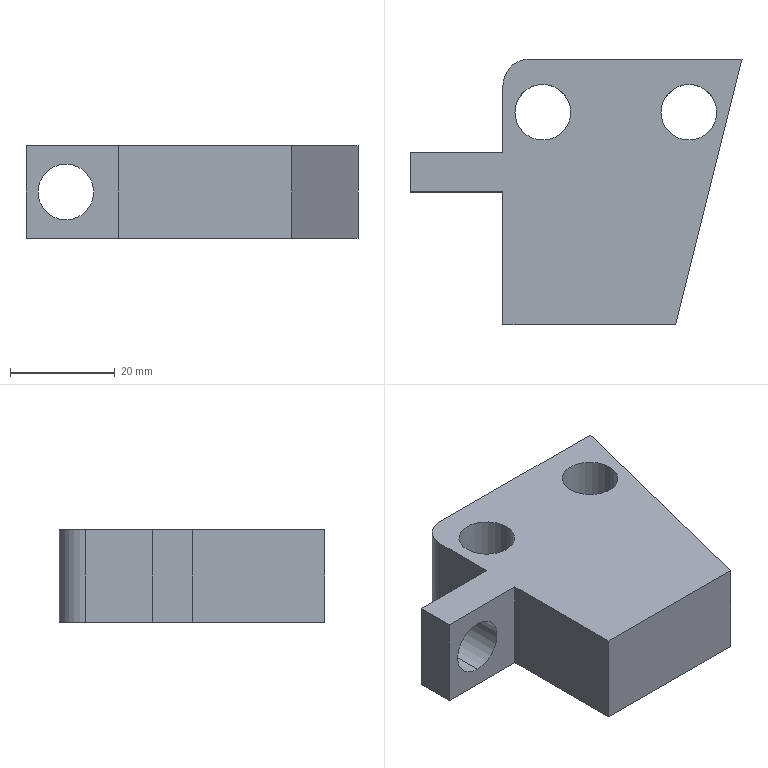Part | SolidWorks | features Extrusion 1, Fillet 1, ICE 1, Scale 1 | 1 solid | 17 faces | box 63.5 x 50.8 x 17.78 mm | volume 34011 mm3 | plane 10 | cylinder 7 | commonest cylinder face diameters 10.668 x6 10.16 x1
STEP:
#1=CARTESIAN_POINT('',(-10.16,25.4,3.556));
#2=VERTEX_POINT('',#1);
#3=CARTESIAN_POINT('',(-10.16,25.4,14.224));
#4=VERTEX_POINT('',#3);
#5=CARTESIAN_POINT('',(-10.16,25.4,8.89));
#6=DIRECTION('',(0.,1.,0.));
#7=DIRECTION('',(-1.,0.,0.));
#8=AXIS2_PLACEMENT_3D('',#5,#6,#7);
#9=CIRCLE('',#8,5.334);
#10=EDGE_CURVE('',#2,#4,#9,.T.);
#11=ORIENTED_EDGE('',*,*,#10,.F.);
#12=CARTESIAN_POINT('',(-10.16,33.02,3.556));
#13=VERTEX_POINT('',#12);
#14=CARTESIAN_POINT('',(-10.16,0.,3.556));
#15=DIRECTION('',(0.,1.,0.));
#16=VECTOR('',#15,1000.);
#17=LINE('',#14,#16);
#18=EDGE_CURVE('',#2,#13,#17,.T.);
#19=ORIENTED_EDGE('',*,*,#18,.T.);
#20=CARTESIAN_POINT('',(-10.16,33.02,14.224));
#21=VERTEX_POINT('',#20);
#22=CARTESIAN_POINT('',(-10.16,33.02,8.89));
#23=DIRECTION('',(0.,1.,0.));
#24=DIRECTION('',(0.,0.,1.));
#25=AXIS2_PLACEMENT_3D('',#22,#23,#24);
#26=CIRCLE('',#25,5.334);
#27=EDGE_CURVE('',#13,#21,#26,.T.);
#28=ORIENTED_EDGE('',*,*,#27,.T.);
#29=CARTESIAN_POINT('',(-10.16,0.,14.224));
#30=DIRECTION('',(0.,1.,0.));
#31=VECTOR('',#30,1000.);
#32=LINE('',#29,#31);
#33=EDGE_CURVE('',#4,#21,#32,.T.);
#34=ORIENTED_EDGE('',*,*,#33,.F.);
#35=EDGE_LOOP('',(#11,#19,#28,#34));
#36=FACE_OUTER_BOUND('',#35,.T.);
#37=CARTESIAN_POINT('',(-10.16,0.,8.89));
#38=DIRECTION('',(0.,1.,0.));
#39=DIRECTION('',(0.,0.,1.));
#40=AXIS2_PLACEMENT_3D('',#37,#38,#39);
#41=CYLINDRICAL_SURFACE('',#40,5.334);
#42=ADVANCED_FACE('',(#36),#41,.F.);
#43=CARTESIAN_POINT('',(30.226,40.64,17.78));
#44=VERTEX_POINT('',#43);
#45=CARTESIAN_POINT('',(40.894,40.64,17.78));
#46=VERTEX_POINT('',#45);
#47=CARTESIAN_POINT('',(35.56,40.64,17.78));
#48=DIRECTION('',(0.,0.,1.));
#49=DIRECTION('',(1.,0.,0.));
#50=AXIS2_PLACEMENT_3D('',#47,#48,#49);
#51=CIRCLE('',#50,5.334);
#52=EDGE_CURVE('',#44,#46,#51,.T.);
#53=ORIENTED_EDGE('',*,*,#52,.T.);
#54=CARTESIAN_POINT('',(40.894,40.64,0.));
#55=VERTEX_POINT('',#54);
#56=CARTESIAN_POINT('',(40.894,40.64,17.78));
#57=DIRECTION('',(0.,0.,-1.));
#58=VECTOR('',#57,1000.);
#59=LINE('',#56,#58);
#60=EDGE_CURVE('',#46,#55,#59,.T.);
#61=ORIENTED_EDGE('',*,*,#60,.T.);
#62=CARTESIAN_POINT('',(30.226,40.64,0.));
#63=VERTEX_POINT('',#62);
#64=CARTESIAN_POINT('',(35.56,40.64,0.));
#65=DIRECTION('',(0.,0.,1.));
#66=DIRECTION('',(1.,0.,0.));
#67=AXIS2_PLACEMENT_3D('',#64,#65,#66);
#68=CIRCLE('',#67,5.334);
#69=EDGE_CURVE('',#63,#55,#68,.T.);
#70=ORIENTED_EDGE('',*,*,#69,.F.);
#71=CARTESIAN_POINT('',(30.226,40.64,17.78));
#72=DIRECTION('',(0.,0.,-1.));
#73=VECTOR('',#72,1000.);
#74=LINE('',#71,#73);
#75=EDGE_CURVE('',#44,#63,#74,.T.);
#76=ORIENTED_EDGE('',*,*,#75,.F.);
#77=EDGE_LOOP('',(#53,#61,#70,#76));
#78=FACE_OUTER_BOUND('',#77,.T.);
#79=CARTESIAN_POINT('',(35.56,40.64,17.78));
#80=DIRECTION('',(0.,0.,-1.));
#81=DIRECTION('',(-1.,0.,0.));
#82=AXIS2_PLACEMENT_3D('',#79,#80,#81);
#83=CYLINDRICAL_SURFACE('',#82,5.334);
#84=ADVANCED_FACE('',(#78),#83,.F.);
#85=CARTESIAN_POINT('',(2.286,40.64,17.78));
#86=VERTEX_POINT('',#85);
#87=CARTESIAN_POINT('',(12.954,40.64,17.78));
#88=VERTEX_POINT('',#87);
#89=CARTESIAN_POINT('',(7.62,40.64,17.78));
#90=DIRECTION('',(0.,0.,1.));
#91=DIRECTION('',(1.,0.,0.));
#92=AXIS2_PLACEMENT_3D('',#89,#90,#91);
#93=CIRCLE('',#92,5.334);
#94=EDGE_CURVE('',#86,#88,#93,.T.);
#95=ORIENTED_EDGE('',*,*,#94,.T.);
#96=CARTESIAN_POINT('',(12.954,40.64,0.));
#97=VERTEX_POINT('',#96);
#98=CARTESIAN_POINT('',(12.954,40.64,17.78));
#99=DIRECTION('',(0.,0.,-1.));
#100=VECTOR('',#99,1000.);
#101=LINE('',#98,#100);
#102=EDGE_CURVE('',#88,#97,#101,.T.);
#103=ORIENTED_EDGE('',*,*,#102,.T.);
#104=CARTESIAN_POINT('',(2.286,40.64,0.));
#105=VERTEX_POINT('',#104);
#106=CARTESIAN_POINT('',(7.62,40.64,0.));
#107=DIRECTION('',(0.,0.,1.));
#108=DIRECTION('',(1.,0.,0.));
#109=AXIS2_PLACEMENT_3D('',#106,#107,#108);
#110=CIRCLE('',#109,5.334);
#111=EDGE_CURVE('',#105,#97,#110,.T.);
#112=ORIENTED_EDGE('',*,*,#111,.F.);
#113=CARTESIAN_POINT('',(2.286,40.64,17.78));
#114=DIRECTION('',(0.,0.,-1.));
#115=VECTOR('',#114,1000.);
#116=LINE('',#113,#115);
#117=EDGE_CURVE('',#86,#105,#116,.T.);
#118=ORIENTED_EDGE('',*,*,#117,.F.);
#119=EDGE_LOOP('',(#95,#103,#112,#118));
#120=FACE_OUTER_BOUND('',#119,.T.);
#121=CARTESIAN_POINT('',(7.62,40.64,17.78));
#122=DIRECTION('',(0.,0.,-1.));
#123=DIRECTION('',(-1.,0.,0.));
#124=AXIS2_PLACEMENT_3D('',#121,#122,#123);
#125=CYLINDRICAL_SURFACE('',#124,5.334);
#126=ADVANCED_FACE('',(#120),#125,.F.);
#127=ORIENTED_EDGE('',*,*,#94,.F.);
#128=CARTESIAN_POINT('',(7.62,40.64,17.78));
#129=DIRECTION('',(0.,0.,1.));
#130=DIRECTION('',(1.,0.,0.));
#131=AXIS2_PLACEMENT_3D('',#128,#129,#130);
#132=CIRCLE('',#131,5.334);
#133=EDGE_CURVE('',#88,#86,#132,.T.);
#134=ORIENTED_EDGE('',*,*,#133,.F.);
#135=EDGE_LOOP('',(#127,#134));
#136=FACE_BOUND('',#135,.T.);
#137=CARTESIAN_POINT('',(45.72,50.8,17.78));
#138=VERTEX_POINT('',#137);
#139=CARTESIAN_POINT('',(5.08,50.8,17.78));
#140=VERTEX_POINT('',#139);
#141=CARTESIAN_POINT('',(0.,50.8,17.78));
#142=DIRECTION('',(-1.,0.,0.));
#143=VECTOR('',#142,1000.);
#144=LINE('',#141,#143);
#145=EDGE_CURVE('',#138,#140,#144,.T.);
#146=ORIENTED_EDGE('',*,*,#145,.T.);
#147=CARTESIAN_POINT('',(0.,45.72,17.78));
#148=VERTEX_POINT('',#147);
#149=CARTESIAN_POINT('',(5.08,45.72,17.78));
#150=DIRECTION('',(0.,0.,1.));
#151=DIRECTION('',(-1.,0.,0.));
#152=AXIS2_PLACEMENT_3D('',#149,#150,#151);
#153=CIRCLE('',#152,5.08);
#154=EDGE_CURVE('',#140,#148,#153,.T.);
#155=ORIENTED_EDGE('',*,*,#154,.T.);
#156=CARTESIAN_POINT('',(0.,33.02,17.78));
#157=VERTEX_POINT('',#156);
#158=CARTESIAN_POINT('',(0.,33.02,17.78));
#159=DIRECTION('',(0.,-1.,0.));
#160=VECTOR('',#159,1000.);
#161=LINE('',#158,#160);
#162=EDGE_CURVE('',#148,#157,#161,.T.);
#163=ORIENTED_EDGE('',*,*,#162,.T.);
#164=CARTESIAN_POINT('',(-17.78,33.02,17.78));
#165=VERTEX_POINT('',#164);
#166=CARTESIAN_POINT('',(-17.78,33.02,17.78));
#167=DIRECTION('',(-1.,0.,0.));
#168=VECTOR('',#167,1000.);
#169=LINE('',#166,#168);
#170=EDGE_CURVE('',#157,#165,#169,.T.);
#171=ORIENTED_EDGE('',*,*,#170,.T.);
#172=CARTESIAN_POINT('',(-17.78,25.4,17.78));
#173=VERTEX_POINT('',#172);
#174=CARTESIAN_POINT('',(-17.78,25.4,17.78));
#175=DIRECTION('',(0.,-1.,0.));
#176=VECTOR('',#175,1000.);
#177=LINE('',#174,#176);
#178=EDGE_CURVE('',#165,#173,#177,.T.);
#179=ORIENTED_EDGE('',*,*,#178,.T.);
#180=CARTESIAN_POINT('',(0.,25.4,17.78));
#181=VERTEX_POINT('',#180);
#182=CARTESIAN_POINT('',(0.,25.4,17.78));
#183=DIRECTION('',(1.,0.,0.));
#184=VECTOR('',#183,1000.);
#185=LINE('',#182,#184);
#186=EDGE_CURVE('',#173,#181,#185,.T.);
#187=ORIENTED_EDGE('',*,*,#186,.T.);
#188=CARTESIAN_POINT('',(0.,0.,17.78));
#189=VERTEX_POINT('',#188);
#190=CARTESIAN_POINT('',(0.,0.,17.78));
#191=DIRECTION('',(0.,-1.,0.));
#192=VECTOR('',#191,1000.);
#193=LINE('',#190,#192);
#194=EDGE_CURVE('',#181,#189,#193,.T.);
#195=ORIENTED_EDGE('',*,*,#194,.T.);
#196=CARTESIAN_POINT('',(33.02,0.,17.78));
#197=VERTEX_POINT('',#196);
#198=CARTESIAN_POINT('',(33.02,0.,17.78));
#199=DIRECTION('',(1.,0.,0.));
#200=VECTOR('',#199,1000.);
#201=LINE('',#198,#200);
#202=EDGE_CURVE('',#189,#197,#201,.T.);
#203=ORIENTED_EDGE('',*,*,#202,.T.);
#204=CARTESIAN_POINT('',(45.72,50.8,17.78));
#205=DIRECTION('',(0.2425,0.9701,0.));
#206=VECTOR('',#205,1000.);
#207=LINE('',#204,#206);
#208=EDGE_CURVE('',#197,#138,#207,.T.);
#209=ORIENTED_EDGE('',*,*,#208,.T.);
#210=EDGE_LOOP('',(#146,#155,#163,#171,#179,#187,#195,#203,#209));
#211=FACE_OUTER_BOUND('',#210,.T.);
#212=ORIENTED_EDGE('',*,*,#52,.F.);
#213=CARTESIAN_POINT('',(35.56,40.64,17.78));
#214=DIRECTION('',(0.,0.,1.));
#215=DIRECTION('',(1.,0.,0.));
#216=AXIS2_PLACEMENT_3D('',#213,#214,#215);
#217=CIRCLE('',#216,5.334);
#218=EDGE_CURVE('',#46,#44,#217,.T.);
#219=ORIENTED_EDGE('',*,*,#218,.F.);
#220=EDGE_LOOP('',(#212,#219));
#221=FACE_BOUND('',#220,.T.);
#222=CARTESIAN_POINT('',(0.,0.,17.78));
#223=DIRECTION('',(0.,0.,-1.));
#224=DIRECTION('',(-1.,0.,0.));
#225=AXIS2_PLACEMENT_3D('',#222,#223,#224);
#226=PLANE('',#225);
#227=ADVANCED_FACE('',(#136,#211,#221),#226,.F.);
#228=ORIENTED_EDGE('',*,*,#111,.T.);
#229=CARTESIAN_POINT('',(7.62,40.64,0.));
#230=DIRECTION('',(0.,0.,1.));
#231=DIRECTION('',(1.,0.,0.));
#232=AXIS2_PLACEMENT_3D('',#229,#230,#231);
#233=CIRCLE('',#232,5.334);
#234=EDGE_CURVE('',#97,#105,#233,.T.);
#235=ORIENTED_EDGE('',*,*,#234,.T.);
#236=EDGE_LOOP('',(#228,#235));
#237=FACE_BOUND('',#236,.T.);
#238=CARTESIAN_POINT('',(0.,45.72,0.));
#239=VERTEX_POINT('',#238);
#240=CARTESIAN_POINT('',(0.,33.02,0.));
#241=VERTEX_POINT('',#240);
#242=CARTESIAN_POINT('',(0.,33.02,0.));
#243=DIRECTION('',(0.,-1.,0.));
#244=VECTOR('',#243,1000.);
#245=LINE('',#242,#244);
#246=EDGE_CURVE('',#239,#241,#245,.T.);
#247=ORIENTED_EDGE('',*,*,#246,.F.);
#248=CARTESIAN_POINT('',(5.08,50.8,0.));
#249=VERTEX_POINT('',#248);
#250=CARTESIAN_POINT('',(5.08,45.72,0.));
#251=DIRECTION('',(0.,0.,-1.));
#252=DIRECTION('',(-1.,0.,0.));
#253=AXIS2_PLACEMENT_3D('',#250,#251,#252);
#254=CIRCLE('',#253,5.08);
#255=EDGE_CURVE('',#239,#249,#254,.T.);
#256=ORIENTED_EDGE('',*,*,#255,.T.);
#257=CARTESIAN_POINT('',(45.72,50.8,0.));
#258=VERTEX_POINT('',#257);
#259=CARTESIAN_POINT('',(0.,50.8,0.));
#260=DIRECTION('',(-1.,0.,0.));
#261=VECTOR('',#260,1000.);
#262=LINE('',#259,#261);
#263=EDGE_CURVE('',#258,#249,#262,.T.);
#264=ORIENTED_EDGE('',*,*,#263,.F.);
#265=CARTESIAN_POINT('',(33.02,0.,0.));
#266=VERTEX_POINT('',#265);
#267=CARTESIAN_POINT('',(45.72,50.8,0.));
#268=DIRECTION('',(0.2425,0.9701,0.));
#269=VECTOR('',#268,1000.);
#270=LINE('',#267,#269);
#271=EDGE_CURVE('',#266,#258,#270,.T.);
#272=ORIENTED_EDGE('',*,*,#271,.F.);
#273=CARTESIAN_POINT('',(0.,0.,0.));
#274=VERTEX_POINT('',#273);
#275=CARTESIAN_POINT('',(33.02,0.,0.));
#276=DIRECTION('',(1.,0.,0.));
#277=VECTOR('',#276,1000.);
#278=LINE('',#275,#277);
#279=EDGE_CURVE('',#274,#266,#278,.T.);
#280=ORIENTED_EDGE('',*,*,#279,.F.);
#281=CARTESIAN_POINT('',(0.,25.4,0.));
#282=VERTEX_POINT('',#281);
#283=CARTESIAN_POINT('',(0.,0.,0.));
#284=DIRECTION('',(0.,-1.,0.));
#285=VECTOR('',#284,1000.);
#286=LINE('',#283,#285);
#287=EDGE_CURVE('',#282,#274,#286,.T.);
#288=ORIENTED_EDGE('',*,*,#287,.F.);
#289=CARTESIAN_POINT('',(-17.78,25.4,0.));
#290=VERTEX_POINT('',#289);
#291=CARTESIAN_POINT('',(0.,25.4,0.));
#292=DIRECTION('',(1.,0.,0.));
#293=VECTOR('',#292,1000.);
#294=LINE('',#291,#293);
#295=EDGE_CURVE('',#290,#282,#294,.T.);
#296=ORIENTED_EDGE('',*,*,#295,.F.);
#297=CARTESIAN_POINT('',(-17.78,33.02,0.));
#298=VERTEX_POINT('',#297);
#299=CARTESIAN_POINT('',(-17.78,25.4,0.));
#300=DIRECTION('',(0.,-1.,0.));
#301=VECTOR('',#300,1000.);
#302=LINE('',#299,#301);
#303=EDGE_CURVE('',#298,#290,#302,.T.);
#304=ORIENTED_EDGE('',*,*,#303,.F.);
#305=CARTESIAN_POINT('',(-17.78,33.02,0.));
#306=DIRECTION('',(-1.,0.,0.));
#307=VECTOR('',#306,1000.);
#308=LINE('',#305,#307);
#309=EDGE_CURVE('',#241,#298,#308,.T.);
#310=ORIENTED_EDGE('',*,*,#309,.F.);
#311=EDGE_LOOP('',(#247,#256,#264,#272,#280,#288,#296,#304,#310));
#312=FACE_OUTER_BOUND('',#311,.T.);
#313=ORIENTED_EDGE('',*,*,#69,.T.);
#314=CARTESIAN_POINT('',(35.56,40.64,0.));
#315=DIRECTION('',(0.,0.,1.));
#316=DIRECTION('',(1.,0.,0.));
#317=AXIS2_PLACEMENT_3D('',#314,#315,#316);
#318=CIRCLE('',#317,5.334);
#319=EDGE_CURVE('',#55,#63,#318,.T.);
#320=ORIENTED_EDGE('',*,*,#319,.T.);
#321=EDGE_LOOP('',(#313,#320));
#322=FACE_BOUND('',#321,.T.);
#323=CARTESIAN_POINT('',(0.,0.,0.));
#324=DIRECTION('',(0.,0.,-1.));
#325=DIRECTION('',(-1.,0.,0.));
#326=AXIS2_PLACEMENT_3D('',#323,#324,#325);
#327=PLANE('',#326);
#328=ADVANCED_FACE('',(#237,#312,#322),#327,.T.);
#329=ORIENTED_EDGE('',*,*,#279,.T.);
#330=CARTESIAN_POINT('',(33.02,0.,17.78));
#331=DIRECTION('',(0.,0.,-1.));
#332=VECTOR('',#331,1000.);
#333=LINE('',#330,#332);
#334=EDGE_CURVE('',#197,#266,#333,.T.);
#335=ORIENTED_EDGE('',*,*,#334,.F.);
#336=ORIENTED_EDGE('',*,*,#202,.F.);
#337=CARTESIAN_POINT('',(0.,0.,17.78));
#338=DIRECTION('',(0.,0.,-1.));
#339=VECTOR('',#338,1000.);
#340=LINE('',#337,#339);
#341=EDGE_CURVE('',#189,#274,#340,.T.);
#342=ORIENTED_EDGE('',*,*,#341,.T.);
#343=EDGE_LOOP('',(#329,#335,#336,#342));
#344=FACE_OUTER_BOUND('',#343,.T.);
#345=CARTESIAN_POINT('',(33.02,0.,17.78));
#346=DIRECTION('',(0.,1.,0.));
#347=DIRECTION('',(-1.,0.,0.));
#348=AXIS2_PLACEMENT_3D('',#345,#346,#347);
#349=PLANE('',#348);
#350=ADVANCED_FACE('',(#344),#349,.F.);
#351=ORIENTED_EDGE('',*,*,#271,.T.);
#352=CARTESIAN_POINT('',(45.72,50.8,17.78));
#353=DIRECTION('',(0.,0.,-1.));
#354=VECTOR('',#353,1000.);
#355=LINE('',#352,#354);
#356=EDGE_CURVE('',#138,#258,#355,.T.);
#357=ORIENTED_EDGE('',*,*,#356,.F.);
#358=ORIENTED_EDGE('',*,*,#208,.F.);
#359=ORIENTED_EDGE('',*,*,#334,.T.);
#360=EDGE_LOOP('',(#351,#357,#358,#359));
#361=FACE_OUTER_BOUND('',#360,.T.);
#362=CARTESIAN_POINT('',(45.72,50.8,17.78));
#363=DIRECTION('',(-0.9701,0.2425,0.));
#364=DIRECTION('',(-0.2425,-0.9701,0.));
#365=AXIS2_PLACEMENT_3D('',#362,#363,#364);
#366=PLANE('',#365);
#367=ADVANCED_FACE('',(#361),#366,.F.);
#368=ORIENTED_EDGE('',*,*,#263,.T.);
#369=CARTESIAN_POINT('',(5.08,50.8,17.78));
#370=DIRECTION('',(0.,0.,1.));
#371=VECTOR('',#370,1000.);
#372=LINE('',#369,#371);
#373=EDGE_CURVE('',#249,#140,#372,.T.);
#374=ORIENTED_EDGE('',*,*,#373,.T.);
#375=ORIENTED_EDGE('',*,*,#145,.F.);
#376=ORIENTED_EDGE('',*,*,#356,.T.);
#377=EDGE_LOOP('',(#368,#374,#375,#376));
#378=FACE_OUTER_BOUND('',#377,.T.);
#379=CARTESIAN_POINT('',(0.,50.8,17.78));
#380=DIRECTION('',(0.,-1.,0.));
#381=DIRECTION('',(0.,0.,-1.));
#382=AXIS2_PLACEMENT_3D('',#379,#380,#381);
#383=PLANE('',#382);
#384=ADVANCED_FACE('',(#378),#383,.F.);
#385=ORIENTED_EDGE('',*,*,#162,.F.);
#386=CARTESIAN_POINT('',(0.,45.72,17.78));
#387=DIRECTION('',(0.,0.,-1.));
#388=VECTOR('',#387,1000.);
#389=LINE('',#386,#388);
#390=EDGE_CURVE('',#148,#239,#389,.T.);
#391=ORIENTED_EDGE('',*,*,#390,.T.);
#392=ORIENTED_EDGE('',*,*,#246,.T.);
#393=CARTESIAN_POINT('',(0.,33.02,17.78));
#394=DIRECTION('',(0.,0.,-1.));
#395=VECTOR('',#394,1000.);
#396=LINE('',#393,#395);
#397=EDGE_CURVE('',#157,#241,#396,.T.);
#398=ORIENTED_EDGE('',*,*,#397,.F.);
#399=EDGE_LOOP('',(#385,#391,#392,#398));
#400=FACE_OUTER_BOUND('',#399,.T.);
#401=CARTESIAN_POINT('',(0.,33.02,17.78));
#402=DIRECTION('',(1.,0.,0.));
#403=DIRECTION('',(0.,0.,-1.));
#404=AXIS2_PLACEMENT_3D('',#401,#402,#403);
#405=PLANE('',#404);
#406=ADVANCED_FACE('',(#400),#405,.F.);
#407=CARTESIAN_POINT('',(-10.16,33.02,8.89));
#408=DIRECTION('',(0.,1.,0.));
#409=DIRECTION('',(0.,0.,1.));
#410=AXIS2_PLACEMENT_3D('',#407,#408,#409);
#411=CIRCLE('',#410,5.334);
#412=EDGE_CURVE('',#21,#13,#411,.T.);
#413=ORIENTED_EDGE('',*,*,#412,.F.);
#414=ORIENTED_EDGE('',*,*,#27,.F.);
#415=EDGE_LOOP('',(#413,#414));
#416=FACE_BOUND('',#415,.T.);
#417=ORIENTED_EDGE('',*,*,#309,.T.);
#418=CARTESIAN_POINT('',(-17.78,33.02,17.78));
#419=DIRECTION('',(0.,0.,-1.));
#420=VECTOR('',#419,1000.);
#421=LINE('',#418,#420);
#422=EDGE_CURVE('',#165,#298,#421,.T.);
#423=ORIENTED_EDGE('',*,*,#422,.F.);
#424=ORIENTED_EDGE('',*,*,#170,.F.);
#425=ORIENTED_EDGE('',*,*,#397,.T.);
#426=EDGE_LOOP('',(#417,#423,#424,#425));
#427=FACE_OUTER_BOUND('',#426,.T.);
#428=CARTESIAN_POINT('',(-17.78,33.02,17.78));
#429=DIRECTION('',(0.,-1.,0.));
#430=DIRECTION('',(0.,0.,-1.));
#431=AXIS2_PLACEMENT_3D('',#428,#429,#430);
#432=PLANE('',#431);
#433=ADVANCED_FACE('',(#416,#427),#432,.F.);
#434=ORIENTED_EDGE('',*,*,#303,.T.);
#435=CARTESIAN_POINT('',(-17.78,25.4,17.78));
#436=DIRECTION('',(0.,0.,-1.));
#437=VECTOR('',#436,1000.);
#438=LINE('',#435,#437);
#439=EDGE_CURVE('',#173,#290,#438,.T.);
#440=ORIENTED_EDGE('',*,*,#439,.F.);
#441=ORIENTED_EDGE('',*,*,#178,.F.);
#442=ORIENTED_EDGE('',*,*,#422,.T.);
#443=EDGE_LOOP('',(#434,#440,#441,#442));
#444=FACE_OUTER_BOUND('',#443,.T.);
#445=CARTESIAN_POINT('',(-17.78,25.4,17.78));
#446=DIRECTION('',(1.,0.,0.));
#447=DIRECTION('',(0.,1.,0.));
#448=AXIS2_PLACEMENT_3D('',#445,#446,#447);
#449=PLANE('',#448);
#450=ADVANCED_FACE('',(#444),#449,.F.);
#451=CARTESIAN_POINT('',(-10.16,25.4,8.89));
#452=DIRECTION('',(0.,1.,0.));
#453=DIRECTION('',(-1.,0.,0.));
#454=AXIS2_PLACEMENT_3D('',#451,#452,#453);
#455=CIRCLE('',#454,5.334);
#456=EDGE_CURVE('',#4,#2,#455,.T.);
#457=ORIENTED_EDGE('',*,*,#456,.T.);
#458=ORIENTED_EDGE('',*,*,#10,.T.);
#459=EDGE_LOOP('',(#457,#458));
#460=FACE_BOUND('',#459,.T.);
#461=ORIENTED_EDGE('',*,*,#295,.T.);
#462=CARTESIAN_POINT('',(0.,25.4,17.78));
#463=DIRECTION('',(0.,0.,-1.));
#464=VECTOR('',#463,1000.);
#465=LINE('',#462,#464);
#466=EDGE_CURVE('',#181,#282,#465,.T.);
#467=ORIENTED_EDGE('',*,*,#466,.F.);
#468=ORIENTED_EDGE('',*,*,#186,.F.);
#469=ORIENTED_EDGE('',*,*,#439,.T.);
#470=EDGE_LOOP('',(#461,#467,#468,#469));
#471=FACE_OUTER_BOUND('',#470,.T.);
#472=CARTESIAN_POINT('',(0.,25.4,17.78));
#473=DIRECTION('',(0.,1.,0.));
#474=DIRECTION('',(-1.,0.,0.));
#475=AXIS2_PLACEMENT_3D('',#472,#473,#474);
#476=PLANE('',#475);
#477=ADVANCED_FACE('',(#460,#471),#476,.F.);
#478=ORIENTED_EDGE('',*,*,#287,.T.);
#479=ORIENTED_EDGE('',*,*,#341,.F.);
#480=ORIENTED_EDGE('',*,*,#194,.F.);
#481=ORIENTED_EDGE('',*,*,#466,.T.);
#482=EDGE_LOOP('',(#478,#479,#480,#481));
#483=FACE_OUTER_BOUND('',#482,.T.);
#484=CARTESIAN_POINT('',(0.,0.,17.78));
#485=DIRECTION('',(1.,0.,0.));
#486=DIRECTION('',(0.,0.,-1.));
#487=AXIS2_PLACEMENT_3D('',#484,#485,#486);
#488=PLANE('',#487);
#489=ADVANCED_FACE('',(#483),#488,.F.);
#490=ORIENTED_EDGE('',*,*,#102,.F.);
#491=ORIENTED_EDGE('',*,*,#133,.T.);
#492=ORIENTED_EDGE('',*,*,#117,.T.);
#493=ORIENTED_EDGE('',*,*,#234,.F.);
#494=EDGE_LOOP('',(#490,#491,#492,#493));
#495=FACE_OUTER_BOUND('',#494,.T.);
#496=CARTESIAN_POINT('',(7.62,40.64,17.78));
#497=DIRECTION('',(0.,0.,-1.));
#498=DIRECTION('',(-1.,0.,0.));
#499=AXIS2_PLACEMENT_3D('',#496,#497,#498);
#500=CYLINDRICAL_SURFACE('',#499,5.334);
#501=ADVANCED_FACE('',(#495),#500,.F.);
#502=ORIENTED_EDGE('',*,*,#60,.F.);
#503=ORIENTED_EDGE('',*,*,#218,.T.);
#504=ORIENTED_EDGE('',*,*,#75,.T.);
#505=ORIENTED_EDGE('',*,*,#319,.F.);
#506=EDGE_LOOP('',(#502,#503,#504,#505));
#507=FACE_OUTER_BOUND('',#506,.T.);
#508=CARTESIAN_POINT('',(35.56,40.64,17.78));
#509=DIRECTION('',(0.,0.,-1.));
#510=DIRECTION('',(-1.,0.,0.));
#511=AXIS2_PLACEMENT_3D('',#508,#509,#510);
#512=CYLINDRICAL_SURFACE('',#511,5.334);
#513=ADVANCED_FACE('',(#507),#512,.F.);
#514=ORIENTED_EDGE('',*,*,#18,.F.);
#515=ORIENTED_EDGE('',*,*,#456,.F.);
#516=ORIENTED_EDGE('',*,*,#33,.T.);
#517=ORIENTED_EDGE('',*,*,#412,.T.);
#518=EDGE_LOOP('',(#514,#515,#516,#517));
#519=FACE_OUTER_BOUND('',#518,.T.);
#520=CARTESIAN_POINT('',(-10.16,0.,8.89));
#521=DIRECTION('',(0.,1.,0.));
#522=DIRECTION('',(0.,0.,1.));
#523=AXIS2_PLACEMENT_3D('',#520,#521,#522);
#524=CYLINDRICAL_SURFACE('',#523,5.334);
#525=ADVANCED_FACE('',(#519),#524,.F.);
#526=ORIENTED_EDGE('',*,*,#154,.F.);
#527=ORIENTED_EDGE('',*,*,#373,.F.);
#528=ORIENTED_EDGE('',*,*,#255,.F.);
#529=ORIENTED_EDGE('',*,*,#390,.F.);
#530=EDGE_LOOP('',(#526,#527,#528,#529));
#531=FACE_OUTER_BOUND('',#530,.T.);
#532=CARTESIAN_POINT('',(5.08,45.72,17.78));
#533=DIRECTION('',(0.,0.,-1.));
#534=DIRECTION('',(-1.,0.,0.));
#535=AXIS2_PLACEMENT_3D('',#532,#533,#534);
#536=CYLINDRICAL_SURFACE('',#535,5.08);
#537=ADVANCED_FACE('',(#531),#536,.T.);
#538=CLOSED_SHELL('',(#42,#84,#126,#227,#328,#350,#367,#384,#406,#433,#450,#477,#489,#501,#513,#525,#537));
#539=MANIFOLD_SOLID_BREP('',#538);
#540=CARTESIAN_POINT('',(0.,0.,0.));
#541=DIRECTION('',(0.,0.,1.));
#542=DIRECTION('',(1.,0.,0.));
#543=AXIS2_PLACEMENT_3D('',#540,#541,#542);
#544=(LENGTH_UNIT()NAMED_UNIT(*)SI_UNIT(.MILLI.,.METRE.));
#545=UNCERTAINTY_MEASURE_WITH_UNIT(LENGTH_MEASURE(0.00001),#544,'','');
#546=(NAMED_UNIT(*)PLANE_ANGLE_UNIT()SI_UNIT($,.RADIAN.));
#547=(NAMED_UNIT(*)SI_UNIT($,.STERADIAN.)SOLID_ANGLE_UNIT());
#548=(GEOMETRIC_REPRESENTATION_CONTEXT(3)GLOBAL_UNCERTAINTY_ASSIGNED_CONTEXT((#545))GLOBAL_UNIT_ASSIGNED_CONTEXT((#544,#546,#547))REPRESENTATION_CONTEXT('',''));
#549=ADVANCED_BREP_SHAPE_REPRESENTATION('',(#539,#543),#548);